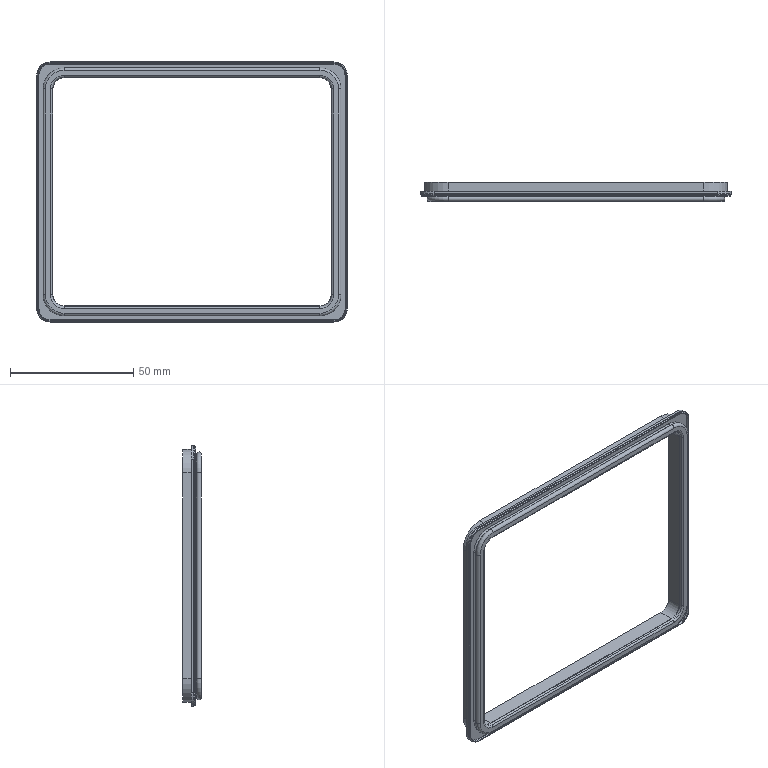Part | STEP file | ZXW735-L-95-06 | 1 solid | 125 faces | box 125.904 x 7.7 x 105.477 mm | volume 15099 mm3 | cylinder 48 | plane 29 | spline 24 | torus 20 | cone 4 | commonest cylinder face diameters 0.2 x12 2 x8 1 x4 1.2 x4 1.4 x4 1.6 x4